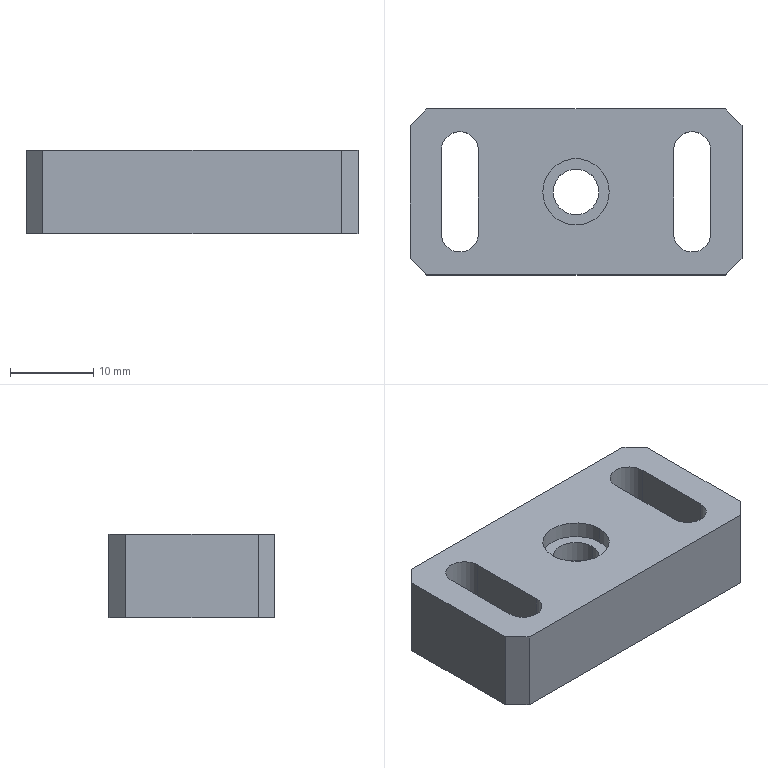Part | STEP file | 11-FG-B06611 | 1 solid | 36 faces | box 40 x 20 x 10 mm | volume 5422 mm3 | plane 22 | cylinder 14 | commonest cylinder face diameters 8 x6 4.5 x4 5.5 x2 10 x2
STEP:
#1=CARTESIAN_POINT('',(25.,-10.,5.4));
#2=VERTEX_POINT('',#1);
#3=CARTESIAN_POINT('',(15.,-10.,5.4));
#4=VERTEX_POINT('',#3);
#5=CARTESIAN_POINT('',(20.,-10.,5.4));
#6=DIRECTION('',(0.,0.,-1.));
#7=DIRECTION('',(-1.,0.,0.));
#8=AXIS2_PLACEMENT_3D('',#5,#6,#7);
#9=CIRCLE('',#8,5.);
#10=EDGE_CURVE('',#2,#4,#9,.T.);
#11=ORIENTED_EDGE('',*,*,#10,.F.);
#12=CARTESIAN_POINT('',(25.,-10.,0.));
#13=VERTEX_POINT('',#12);
#14=CARTESIAN_POINT('',(25.,-10.,0.));
#15=DIRECTION('',(0.,0.,-1.));
#16=VECTOR('',#15,1000.);
#17=LINE('',#14,#16);
#18=EDGE_CURVE('',#2,#13,#17,.T.);
#19=ORIENTED_EDGE('',*,*,#18,.T.);
#20=CARTESIAN_POINT('',(15.,-10.,0.));
#21=VERTEX_POINT('',#20);
#22=CARTESIAN_POINT('',(20.,-10.,0.));
#23=DIRECTION('',(0.,0.,-1.));
#24=DIRECTION('',(-1.,0.,0.));
#25=AXIS2_PLACEMENT_3D('',#22,#23,#24);
#26=CIRCLE('',#25,5.);
#27=EDGE_CURVE('',#13,#21,#26,.T.);
#28=ORIENTED_EDGE('',*,*,#27,.T.);
#29=CARTESIAN_POINT('',(15.,-10.,0.));
#30=DIRECTION('',(0.,0.,-1.));
#31=VECTOR('',#30,1000.);
#32=LINE('',#29,#31);
#33=EDGE_CURVE('',#4,#21,#32,.T.);
#34=ORIENTED_EDGE('',*,*,#33,.F.);
#35=EDGE_LOOP('',(#11,#19,#28,#34));
#36=FACE_OUTER_BOUND('',#35,.T.);
#37=CARTESIAN_POINT('',(20.,-10.,0.));
#38=DIRECTION('',(0.,0.,-1.));
#39=DIRECTION('',(-1.,0.,0.));
#40=AXIS2_PLACEMENT_3D('',#37,#38,#39);
#41=CYLINDRICAL_SURFACE('',#40,5.);
#42=ADVANCED_FACE('',(#36),#41,.F.);
#43=CARTESIAN_POINT('',(17.25,-10.,8.));
#44=VERTEX_POINT('',#43);
#45=CARTESIAN_POINT('',(22.75,-10.,8.));
#46=VERTEX_POINT('',#45);
#47=CARTESIAN_POINT('',(20.,-10.,8.));
#48=DIRECTION('',(0.,0.,1.));
#49=DIRECTION('',(1.,0.,0.));
#50=AXIS2_PLACEMENT_3D('',#47,#48,#49);
#51=CIRCLE('',#50,2.75);
#52=EDGE_CURVE('',#44,#46,#51,.T.);
#53=ORIENTED_EDGE('',*,*,#52,.T.);
#54=CARTESIAN_POINT('',(22.75,-10.,5.4));
#55=VERTEX_POINT('',#54);
#56=CARTESIAN_POINT('',(22.75,-10.,0.));
#57=DIRECTION('',(0.,0.,-1.));
#58=VECTOR('',#57,1000.);
#59=LINE('',#56,#58);
#60=EDGE_CURVE('',#46,#55,#59,.T.);
#61=ORIENTED_EDGE('',*,*,#60,.T.);
#62=CARTESIAN_POINT('',(17.25,-10.,5.4));
#63=VERTEX_POINT('',#62);
#64=CARTESIAN_POINT('',(20.,-10.,5.4));
#65=DIRECTION('',(0.,0.,-1.));
#66=DIRECTION('',(-1.,0.,0.));
#67=AXIS2_PLACEMENT_3D('',#64,#65,#66);
#68=CIRCLE('',#67,2.75);
#69=EDGE_CURVE('',#55,#63,#68,.T.);
#70=ORIENTED_EDGE('',*,*,#69,.T.);
#71=CARTESIAN_POINT('',(17.25,-10.,0.));
#72=DIRECTION('',(0.,0.,-1.));
#73=VECTOR('',#72,1000.);
#74=LINE('',#71,#73);
#75=EDGE_CURVE('',#44,#63,#74,.T.);
#76=ORIENTED_EDGE('',*,*,#75,.F.);
#77=EDGE_LOOP('',(#53,#61,#70,#76));
#78=FACE_OUTER_BOUND('',#77,.T.);
#79=CARTESIAN_POINT('',(20.,-10.,0.));
#80=DIRECTION('',(0.,0.,-1.));
#81=DIRECTION('',(-1.,0.,0.));
#82=AXIS2_PLACEMENT_3D('',#79,#80,#81);
#83=CYLINDRICAL_SURFACE('',#82,2.75);
#84=ADVANCED_FACE('',(#78),#83,.F.);
#85=CARTESIAN_POINT('',(16.,-10.,8.));
#86=VERTEX_POINT('',#85);
#87=CARTESIAN_POINT('',(24.,-10.,8.));
#88=VERTEX_POINT('',#87);
#89=CARTESIAN_POINT('',(20.,-10.,8.));
#90=DIRECTION('',(0.,0.,1.));
#91=DIRECTION('',(1.,0.,0.));
#92=AXIS2_PLACEMENT_3D('',#89,#90,#91);
#93=CIRCLE('',#92,4.);
#94=EDGE_CURVE('',#86,#88,#93,.T.);
#95=ORIENTED_EDGE('',*,*,#94,.F.);
#96=CARTESIAN_POINT('',(16.,-10.,10.));
#97=VERTEX_POINT('',#96);
#98=CARTESIAN_POINT('',(16.,-10.,8.));
#99=DIRECTION('',(0.,0.,1.));
#100=VECTOR('',#99,1000.);
#101=LINE('',#98,#100);
#102=EDGE_CURVE('',#86,#97,#101,.T.);
#103=ORIENTED_EDGE('',*,*,#102,.T.);
#104=CARTESIAN_POINT('',(24.,-10.,10.));
#105=VERTEX_POINT('',#104);
#106=CARTESIAN_POINT('',(20.,-10.,10.));
#107=DIRECTION('',(0.,0.,1.));
#108=DIRECTION('',(1.,0.,0.));
#109=AXIS2_PLACEMENT_3D('',#106,#107,#108);
#110=CIRCLE('',#109,4.);
#111=EDGE_CURVE('',#97,#105,#110,.T.);
#112=ORIENTED_EDGE('',*,*,#111,.T.);
#113=CARTESIAN_POINT('',(24.,-10.,8.));
#114=DIRECTION('',(0.,0.,1.));
#115=VECTOR('',#114,1000.);
#116=LINE('',#113,#115);
#117=EDGE_CURVE('',#88,#105,#116,.T.);
#118=ORIENTED_EDGE('',*,*,#117,.F.);
#119=EDGE_LOOP('',(#95,#103,#112,#118));
#120=FACE_OUTER_BOUND('',#119,.T.);
#121=CARTESIAN_POINT('',(20.,-10.,8.));
#122=DIRECTION('',(0.,0.,1.));
#123=DIRECTION('',(1.,0.,0.));
#124=AXIS2_PLACEMENT_3D('',#121,#122,#123);
#125=CYLINDRICAL_SURFACE('',#124,4.);
#126=ADVANCED_FACE('',(#120),#125,.F.);
#127=CARTESIAN_POINT('',(3.75,-15.,5.));
#128=VERTEX_POINT('',#127);
#129=CARTESIAN_POINT('',(8.25,-15.,5.));
#130=VERTEX_POINT('',#129);
#131=CARTESIAN_POINT('',(6.,-15.,5.));
#132=DIRECTION('',(0.,0.,1.));
#133=DIRECTION('',(-1.,0.,0.));
#134=AXIS2_PLACEMENT_3D('',#131,#132,#133);
#135=CIRCLE('',#134,2.25);
#136=EDGE_CURVE('',#128,#130,#135,.T.);
#137=ORIENTED_EDGE('',*,*,#136,.F.);
#138=CARTESIAN_POINT('',(3.75,-15.,10.));
#139=VERTEX_POINT('',#138);
#140=CARTESIAN_POINT('',(3.75,-15.,23.));
#141=DIRECTION('',(0.,0.,-1.));
#142=VECTOR('',#141,1000.);
#143=LINE('',#140,#142);
#144=EDGE_CURVE('',#139,#128,#143,.T.);
#145=ORIENTED_EDGE('',*,*,#144,.F.);
#146=CARTESIAN_POINT('',(8.25,-15.,10.));
#147=VERTEX_POINT('',#146);
#148=CARTESIAN_POINT('',(6.,-15.,10.));
#149=DIRECTION('',(0.,0.,1.));
#150=DIRECTION('',(1.,0.,0.));
#151=AXIS2_PLACEMENT_3D('',#148,#149,#150);
#152=CIRCLE('',#151,2.25);
#153=EDGE_CURVE('',#139,#147,#152,.T.);
#154=ORIENTED_EDGE('',*,*,#153,.T.);
#155=CARTESIAN_POINT('',(8.25,-15.,23.));
#156=DIRECTION('',(0.,0.,-1.));
#157=VECTOR('',#156,1000.);
#158=LINE('',#155,#157);
#159=EDGE_CURVE('',#147,#130,#158,.T.);
#160=ORIENTED_EDGE('',*,*,#159,.T.);
#161=EDGE_LOOP('',(#137,#145,#154,#160));
#162=FACE_OUTER_BOUND('',#161,.T.);
#163=CARTESIAN_POINT('',(6.,-15.,23.));
#164=DIRECTION('',(0.,0.,-1.));
#165=DIRECTION('',(-1.,0.,0.));
#166=AXIS2_PLACEMENT_3D('',#163,#164,#165);
#167=CYLINDRICAL_SURFACE('',#166,2.25);
#168=ADVANCED_FACE('',(#162),#167,.F.);
#169=CARTESIAN_POINT('',(8.25,-5.,5.));
#170=VERTEX_POINT('',#169);
#171=CARTESIAN_POINT('',(8.25,-15.,5.));
#172=DIRECTION('',(0.,1.,0.));
#173=VECTOR('',#172,1000.);
#174=LINE('',#171,#173);
#175=EDGE_CURVE('',#130,#170,#174,.T.);
#176=ORIENTED_EDGE('',*,*,#175,.F.);
#177=ORIENTED_EDGE('',*,*,#159,.F.);
#178=CARTESIAN_POINT('',(8.25,-5.,10.));
#179=VERTEX_POINT('',#178);
#180=CARTESIAN_POINT('',(8.25,-20.,10.));
#181=DIRECTION('',(0.,1.,0.));
#182=VECTOR('',#181,1000.);
#183=LINE('',#180,#182);
#184=EDGE_CURVE('',#147,#179,#183,.T.);
#185=ORIENTED_EDGE('',*,*,#184,.T.);
#186=CARTESIAN_POINT('',(8.25,-5.,23.));
#187=DIRECTION('',(0.,0.,-1.));
#188=VECTOR('',#187,1000.);
#189=LINE('',#186,#188);
#190=EDGE_CURVE('',#179,#170,#189,.T.);
#191=ORIENTED_EDGE('',*,*,#190,.T.);
#192=EDGE_LOOP('',(#176,#177,#185,#191));
#193=FACE_OUTER_BOUND('',#192,.T.);
#194=CARTESIAN_POINT('',(8.25,-15.,23.));
#195=DIRECTION('',(1.,0.,0.));
#196=DIRECTION('',(0.,1.,0.));
#197=AXIS2_PLACEMENT_3D('',#194,#195,#196);
#198=PLANE('',#197);
#199=ADVANCED_FACE('',(#193),#198,.F.);
#200=CARTESIAN_POINT('',(3.75,-5.,5.));
#201=VERTEX_POINT('',#200);
#202=CARTESIAN_POINT('',(6.,-5.,5.));
#203=DIRECTION('',(0.,0.,1.));
#204=DIRECTION('',(-1.,0.,0.));
#205=AXIS2_PLACEMENT_3D('',#202,#203,#204);
#206=CIRCLE('',#205,2.25);
#207=EDGE_CURVE('',#170,#201,#206,.T.);
#208=ORIENTED_EDGE('',*,*,#207,.F.);
#209=ORIENTED_EDGE('',*,*,#190,.F.);
#210=CARTESIAN_POINT('',(3.75,-5.,10.));
#211=VERTEX_POINT('',#210);
#212=CARTESIAN_POINT('',(6.,-5.,10.));
#213=DIRECTION('',(0.,0.,1.));
#214=DIRECTION('',(1.,0.,0.));
#215=AXIS2_PLACEMENT_3D('',#212,#213,#214);
#216=CIRCLE('',#215,2.25);
#217=EDGE_CURVE('',#179,#211,#216,.T.);
#218=ORIENTED_EDGE('',*,*,#217,.T.);
#219=CARTESIAN_POINT('',(3.75,-5.,23.));
#220=DIRECTION('',(0.,0.,-1.));
#221=VECTOR('',#220,1000.);
#222=LINE('',#219,#221);
#223=EDGE_CURVE('',#211,#201,#222,.T.);
#224=ORIENTED_EDGE('',*,*,#223,.T.);
#225=EDGE_LOOP('',(#208,#209,#218,#224));
#226=FACE_OUTER_BOUND('',#225,.T.);
#227=CARTESIAN_POINT('',(6.,-5.,23.));
#228=DIRECTION('',(0.,0.,-1.));
#229=DIRECTION('',(-1.,0.,0.));
#230=AXIS2_PLACEMENT_3D('',#227,#228,#229);
#231=CYLINDRICAL_SURFACE('',#230,2.25);
#232=ADVANCED_FACE('',(#226),#231,.F.);
#233=CARTESIAN_POINT('',(3.75,-15.,5.));
#234=DIRECTION('',(0.,-1.,0.));
#235=VECTOR('',#234,1000.);
#236=LINE('',#233,#235);
#237=EDGE_CURVE('',#201,#128,#236,.T.);
#238=ORIENTED_EDGE('',*,*,#237,.F.);
#239=ORIENTED_EDGE('',*,*,#223,.F.);
#240=CARTESIAN_POINT('',(3.75,-20.,10.));
#241=DIRECTION('',(0.,-1.,0.));
#242=VECTOR('',#241,1000.);
#243=LINE('',#240,#242);
#244=EDGE_CURVE('',#211,#139,#243,.T.);
#245=ORIENTED_EDGE('',*,*,#244,.T.);
#246=ORIENTED_EDGE('',*,*,#144,.T.);
#247=EDGE_LOOP('',(#238,#239,#245,#246));
#248=FACE_OUTER_BOUND('',#247,.T.);
#249=CARTESIAN_POINT('',(3.75,-15.,23.));
#250=DIRECTION('',(-1.,0.,0.));
#251=DIRECTION('',(0.,-1.,0.));
#252=AXIS2_PLACEMENT_3D('',#249,#250,#251);
#253=PLANE('',#252);
#254=ADVANCED_FACE('',(#248),#253,.F.);
#255=CARTESIAN_POINT('',(36.25,-15.,10.));
#256=VERTEX_POINT('',#255);
#257=CARTESIAN_POINT('',(36.25,-15.,5.));
#258=VERTEX_POINT('',#257);
#259=CARTESIAN_POINT('',(36.25,-15.,23.));
#260=DIRECTION('',(0.,0.,-1.));
#261=VECTOR('',#260,1000.);
#262=LINE('',#259,#261);
#263=EDGE_CURVE('',#256,#258,#262,.T.);
#264=ORIENTED_EDGE('',*,*,#263,.T.);
#265=CARTESIAN_POINT('',(31.75,-15.,5.));
#266=VERTEX_POINT('',#265);
#267=CARTESIAN_POINT('',(34.,-15.,5.));
#268=DIRECTION('',(0.,0.,-1.));
#269=DIRECTION('',(-1.,0.,0.));
#270=AXIS2_PLACEMENT_3D('',#267,#268,#269);
#271=CIRCLE('',#270,2.25);
#272=EDGE_CURVE('',#258,#266,#271,.T.);
#273=ORIENTED_EDGE('',*,*,#272,.T.);
#274=CARTESIAN_POINT('',(31.75,-15.,10.));
#275=VERTEX_POINT('',#274);
#276=CARTESIAN_POINT('',(31.75,-15.,23.));
#277=DIRECTION('',(0.,0.,-1.));
#278=VECTOR('',#277,1000.);
#279=LINE('',#276,#278);
#280=EDGE_CURVE('',#275,#266,#279,.T.);
#281=ORIENTED_EDGE('',*,*,#280,.F.);
#282=CARTESIAN_POINT('',(34.,-15.,10.));
#283=DIRECTION('',(0.,0.,-1.));
#284=DIRECTION('',(1.,0.,0.));
#285=AXIS2_PLACEMENT_3D('',#282,#283,#284);
#286=CIRCLE('',#285,2.25);
#287=EDGE_CURVE('',#256,#275,#286,.T.);
#288=ORIENTED_EDGE('',*,*,#287,.F.);
#289=EDGE_LOOP('',(#264,#273,#281,#288));
#290=FACE_OUTER_BOUND('',#289,.T.);
#291=CARTESIAN_POINT('',(34.,-15.,23.));
#292=DIRECTION('',(0.,0.,-1.));
#293=DIRECTION('',(-1.,0.,0.));
#294=AXIS2_PLACEMENT_3D('',#291,#292,#293);
#295=CYLINDRICAL_SURFACE('',#294,2.25);
#296=ADVANCED_FACE('',(#290),#295,.F.);
#297=CARTESIAN_POINT('',(36.25,-5.,10.));
#298=VERTEX_POINT('',#297);
#299=CARTESIAN_POINT('',(36.25,-5.,5.));
#300=VERTEX_POINT('',#299);
#301=CARTESIAN_POINT('',(36.25,-5.,23.));
#302=DIRECTION('',(0.,0.,-1.));
#303=VECTOR('',#302,1000.);
#304=LINE('',#301,#303);
#305=EDGE_CURVE('',#298,#300,#304,.T.);
#306=ORIENTED_EDGE('',*,*,#305,.T.);
#307=CARTESIAN_POINT('',(36.25,-15.,5.));
#308=DIRECTION('',(0.,-1.,0.));
#309=VECTOR('',#308,1000.);
#310=LINE('',#307,#309);
#311=EDGE_CURVE('',#300,#258,#310,.T.);
#312=ORIENTED_EDGE('',*,*,#311,.T.);
#313=ORIENTED_EDGE('',*,*,#263,.F.);
#314=CARTESIAN_POINT('',(36.25,-20.,10.));
#315=DIRECTION('',(0.,-1.,0.));
#316=VECTOR('',#315,1000.);
#317=LINE('',#314,#316);
#318=EDGE_CURVE('',#298,#256,#317,.T.);
#319=ORIENTED_EDGE('',*,*,#318,.F.);
#320=EDGE_LOOP('',(#306,#312,#313,#319));
#321=FACE_OUTER_BOUND('',#320,.T.);
#322=CARTESIAN_POINT('',(36.25,-15.,23.));
#323=DIRECTION('',(-1.,0.,0.));
#324=DIRECTION('',(0.,-1.,0.));
#325=AXIS2_PLACEMENT_3D('',#322,#323,#324);
#326=PLANE('',#325);
#327=ADVANCED_FACE('',(#321),#326,.T.);
#328=CARTESIAN_POINT('',(31.75,-5.,10.));
#329=VERTEX_POINT('',#328);
#330=CARTESIAN_POINT('',(31.75,-5.,5.));
#331=VERTEX_POINT('',#330);
#332=CARTESIAN_POINT('',(31.75,-5.,23.));
#333=DIRECTION('',(0.,0.,-1.));
#334=VECTOR('',#333,1000.);
#335=LINE('',#332,#334);
#336=EDGE_CURVE('',#329,#331,#335,.T.);
#337=ORIENTED_EDGE('',*,*,#336,.T.);
#338=CARTESIAN_POINT('',(34.,-5.,5.));
#339=DIRECTION('',(0.,0.,-1.));
#340=DIRECTION('',(-1.,0.,0.));
#341=AXIS2_PLACEMENT_3D('',#338,#339,#340);
#342=CIRCLE('',#341,2.25);
#343=EDGE_CURVE('',#331,#300,#342,.T.);
#344=ORIENTED_EDGE('',*,*,#343,.T.);
#345=ORIENTED_EDGE('',*,*,#305,.F.);
#346=CARTESIAN_POINT('',(34.,-5.,10.));
#347=DIRECTION('',(0.,0.,-1.));
#348=DIRECTION('',(1.,0.,0.));
#349=AXIS2_PLACEMENT_3D('',#346,#347,#348);
#350=CIRCLE('',#349,2.25);
#351=EDGE_CURVE('',#329,#298,#350,.T.);
#352=ORIENTED_EDGE('',*,*,#351,.F.);
#353=EDGE_LOOP('',(#337,#344,#345,#352));
#354=FACE_OUTER_BOUND('',#353,.T.);
#355=CARTESIAN_POINT('',(34.,-5.,23.));
#356=DIRECTION('',(0.,0.,-1.));
#357=DIRECTION('',(-1.,0.,0.));
#358=AXIS2_PLACEMENT_3D('',#355,#356,#357);
#359=CYLINDRICAL_SURFACE('',#358,2.25);
#360=ADVANCED_FACE('',(#354),#359,.F.);
#361=ORIENTED_EDGE('',*,*,#280,.T.);
#362=CARTESIAN_POINT('',(31.75,-15.,5.));
#363=DIRECTION('',(0.,1.,0.));
#364=VECTOR('',#363,1000.);
#365=LINE('',#362,#364);
#366=EDGE_CURVE('',#266,#331,#365,.T.);
#367=ORIENTED_EDGE('',*,*,#366,.T.);
#368=ORIENTED_EDGE('',*,*,#336,.F.);
#369=CARTESIAN_POINT('',(31.75,-20.,10.));
#370=DIRECTION('',(0.,1.,0.));
#371=VECTOR('',#370,1000.);
#372=LINE('',#369,#371);
#373=EDGE_CURVE('',#275,#329,#372,.T.);
#374=ORIENTED_EDGE('',*,*,#373,.F.);
#375=EDGE_LOOP('',(#361,#367,#368,#374));
#376=FACE_OUTER_BOUND('',#375,.T.);
#377=CARTESIAN_POINT('',(31.75,-15.,23.));
#378=DIRECTION('',(1.,0.,0.));
#379=DIRECTION('',(0.,1.,0.));
#380=AXIS2_PLACEMENT_3D('',#377,#378,#379);
#381=PLANE('',#380);
#382=ADVANCED_FACE('',(#376),#381,.T.);
#383=ORIENTED_EDGE('',*,*,#153,.F.);
#384=ORIENTED_EDGE('',*,*,#244,.F.);
#385=ORIENTED_EDGE('',*,*,#217,.F.);
#386=ORIENTED_EDGE('',*,*,#184,.F.);
#387=EDGE_LOOP('',(#383,#384,#385,#386));
#388=FACE_BOUND('',#387,.T.);
#389=CARTESIAN_POINT('',(20.,-10.,10.));
#390=DIRECTION('',(0.,0.,1.));
#391=DIRECTION('',(1.,0.,0.));
#392=AXIS2_PLACEMENT_3D('',#389,#390,#391);
#393=CIRCLE('',#392,4.);
#394=EDGE_CURVE('',#105,#97,#393,.T.);
#395=ORIENTED_EDGE('',*,*,#394,.F.);
#396=ORIENTED_EDGE('',*,*,#111,.F.);
#397=EDGE_LOOP('',(#395,#396));
#398=FACE_BOUND('',#397,.T.);
#399=CARTESIAN_POINT('',(0.,-2.,10.));
#400=VERTEX_POINT('',#399);
#401=CARTESIAN_POINT('',(0.,-18.,10.));
#402=VERTEX_POINT('',#401);
#403=CARTESIAN_POINT('',(0.,0.,10.));
#404=DIRECTION('',(0.,-1.,0.));
#405=VECTOR('',#404,1000.);
#406=LINE('',#403,#405);
#407=EDGE_CURVE('',#400,#402,#406,.T.);
#408=ORIENTED_EDGE('',*,*,#407,.T.);
#409=CARTESIAN_POINT('',(2.,-20.,10.));
#410=VERTEX_POINT('',#409);
#411=CARTESIAN_POINT('',(1.,-19.,10.));
#412=DIRECTION('',(0.7071,-0.7071,0.));
#413=VECTOR('',#412,1000.);
#414=LINE('',#411,#413);
#415=EDGE_CURVE('',#402,#410,#414,.T.);
#416=ORIENTED_EDGE('',*,*,#415,.T.);
#417=CARTESIAN_POINT('',(38.,-20.,10.));
#418=VERTEX_POINT('',#417);
#419=CARTESIAN_POINT('',(0.,-20.,10.));
#420=DIRECTION('',(1.,0.,0.));
#421=VECTOR('',#420,1000.);
#422=LINE('',#419,#421);
#423=EDGE_CURVE('',#410,#418,#422,.T.);
#424=ORIENTED_EDGE('',*,*,#423,.T.);
#425=CARTESIAN_POINT('',(40.,-18.,10.));
#426=VERTEX_POINT('',#425);
#427=CARTESIAN_POINT('',(19.,-39.,10.));
#428=DIRECTION('',(0.7071,0.7071,0.));
#429=VECTOR('',#428,1000.);
#430=LINE('',#427,#429);
#431=EDGE_CURVE('',#418,#426,#430,.T.);
#432=ORIENTED_EDGE('',*,*,#431,.T.);
#433=CARTESIAN_POINT('',(40.,-2.,10.));
#434=VERTEX_POINT('',#433);
#435=CARTESIAN_POINT('',(40.,0.,10.));
#436=DIRECTION('',(0.,1.,0.));
#437=VECTOR('',#436,1000.);
#438=LINE('',#435,#437);
#439=EDGE_CURVE('',#426,#434,#438,.T.);
#440=ORIENTED_EDGE('',*,*,#439,.T.);
#441=CARTESIAN_POINT('',(38.,0.,10.));
#442=VERTEX_POINT('',#441);
#443=CARTESIAN_POINT('',(29.,9.,10.));
#444=DIRECTION('',(-0.7071,0.7071,0.));
#445=VECTOR('',#444,1000.);
#446=LINE('',#443,#445);
#447=EDGE_CURVE('',#434,#442,#446,.T.);
#448=ORIENTED_EDGE('',*,*,#447,.T.);
#449=CARTESIAN_POINT('',(2.,0.,10.));
#450=VERTEX_POINT('',#449);
#451=CARTESIAN_POINT('',(0.,0.,10.));
#452=DIRECTION('',(-1.,0.,0.));
#453=VECTOR('',#452,1000.);
#454=LINE('',#451,#453);
#455=EDGE_CURVE('',#442,#450,#454,.T.);
#456=ORIENTED_EDGE('',*,*,#455,.T.);
#457=CARTESIAN_POINT('',(-9.,-11.,10.));
#458=DIRECTION('',(-0.7071,-0.7071,0.));
#459=VECTOR('',#458,1000.);
#460=LINE('',#457,#459);
#461=EDGE_CURVE('',#450,#400,#460,.T.);
#462=ORIENTED_EDGE('',*,*,#461,.T.);
#463=EDGE_LOOP('',(#408,#416,#424,#432,#440,#448,#456,#462));
#464=FACE_OUTER_BOUND('',#463,.T.);
#465=ORIENTED_EDGE('',*,*,#318,.T.);
#466=ORIENTED_EDGE('',*,*,#287,.T.);
#467=ORIENTED_EDGE('',*,*,#373,.T.);
#468=ORIENTED_EDGE('',*,*,#351,.T.);
#469=EDGE_LOOP('',(#465,#466,#467,#468));
#470=FACE_BOUND('',#469,.T.);
#471=CARTESIAN_POINT('',(0.,-20.,10.));
#472=DIRECTION('',(0.,0.,1.));
#473=DIRECTION('',(1.,0.,0.));
#474=AXIS2_PLACEMENT_3D('',#471,#472,#473);
#475=PLANE('',#474);
#476=ADVANCED_FACE('',(#388,#398,#464,#470),#475,.T.);
#477=CARTESIAN_POINT('',(10.,-5.,0.));
#478=VERTEX_POINT('',#477);
#479=CARTESIAN_POINT('',(10.,-15.,0.));
#480=VERTEX_POINT('',#479);
#481=CARTESIAN_POINT('',(10.,-5.,0.));
#482=DIRECTION('',(0.,-1.,0.));
#483=VECTOR('',#482,1000.);
#484=LINE('',#481,#483);
#485=EDGE_CURVE('',#478,#480,#484,.T.);
#486=ORIENTED_EDGE('',*,*,#485,.F.);
#487=CARTESIAN_POINT('',(2.,-5.,0.));
#488=VERTEX_POINT('',#487);
#489=CARTESIAN_POINT('',(6.,-5.,0.));
#490=DIRECTION('',(0.,0.,-1.));
#491=DIRECTION('',(-1.,0.,0.));
#492=AXIS2_PLACEMENT_3D('',#489,#490,#491);
#493=CIRCLE('',#492,4.);
#494=EDGE_CURVE('',#488,#478,#493,.T.);
#495=ORIENTED_EDGE('',*,*,#494,.F.);
#496=CARTESIAN_POINT('',(2.,-15.,0.));
#497=VERTEX_POINT('',#496);
#498=CARTESIAN_POINT('',(2.,-5.,0.));
#499=DIRECTION('',(0.,1.,0.));
#500=VECTOR('',#499,1000.);
#501=LINE('',#498,#500);
#502=EDGE_CURVE('',#497,#488,#501,.T.);
#503=ORIENTED_EDGE('',*,*,#502,.F.);
#504=CARTESIAN_POINT('',(6.,-15.,0.));
#505=DIRECTION('',(0.,0.,-1.));
#506=DIRECTION('',(-1.,0.,0.));
#507=AXIS2_PLACEMENT_3D('',#504,#505,#506);
#508=CIRCLE('',#507,4.);
#509=EDGE_CURVE('',#480,#497,#508,.T.);
#510=ORIENTED_EDGE('',*,*,#509,.F.);
#511=EDGE_LOOP('',(#486,#495,#503,#510));
#512=FACE_BOUND('',#511,.T.);
#513=CARTESIAN_POINT('',(38.,-5.,0.));
#514=VERTEX_POINT('',#513);
#515=CARTESIAN_POINT('',(38.,-15.,0.));
#516=VERTEX_POINT('',#515);
#517=CARTESIAN_POINT('',(38.,-5.,0.));
#518=DIRECTION('',(0.,-1.,0.));
#519=VECTOR('',#518,1000.);
#520=LINE('',#517,#519);
#521=EDGE_CURVE('',#514,#516,#520,.T.);
#522=ORIENTED_EDGE('',*,*,#521,.F.);
#523=CARTESIAN_POINT('',(30.,-5.,0.));
#524=VERTEX_POINT('',#523);
#525=CARTESIAN_POINT('',(34.,-5.,0.));
#526=DIRECTION('',(0.,0.,-1.));
#527=DIRECTION('',(-1.,0.,0.));
#528=AXIS2_PLACEMENT_3D('',#525,#526,#527);
#529=CIRCLE('',#528,4.);
#530=EDGE_CURVE('',#524,#514,#529,.T.);
#531=ORIENTED_EDGE('',*,*,#530,.F.);
#532=CARTESIAN_POINT('',(30.,-15.,0.));
#533=VERTEX_POINT('',#532);
#534=CARTESIAN_POINT('',(30.,-5.,0.));
#535=DIRECTION('',(0.,1.,0.));
#536=VECTOR('',#535,1000.);
#537=LINE('',#534,#536);
#538=EDGE_CURVE('',#533,#524,#537,.T.);
#539=ORIENTED_EDGE('',*,*,#538,.F.);
#540=CARTESIAN_POINT('',(34.,-15.,0.));
#541=DIRECTION('',(0.,0.,-1.));
#542=DIRECTION('',(-1.,0.,0.));
#543=AXIS2_PLACEMENT_3D('',#540,#541,#542);
#544=CIRCLE('',#543,4.);
#545=EDGE_CURVE('',#516,#533,#544,.T.);
#546=ORIENTED_EDGE('',*,*,#545,.F.);
#547=EDGE_LOOP('',(#522,#531,#539,#546));
#548=FACE_BOUND('',#547,.T.);
#549=CARTESIAN_POINT('',(2.,-20.,0.));
#550=VERTEX_POINT('',#549);
#551=CARTESIAN_POINT('',(38.,-20.,0.));
#552=VERTEX_POINT('',#551);
#553=CARTESIAN_POINT('',(0.,-20.,0.));
#554=DIRECTION('',(1.,0.,0.));
#555=VECTOR('',#554,1000.);
#556=LINE('',#553,#555);
#557=EDGE_CURVE('',#550,#552,#556,.T.);
#558=ORIENTED_EDGE('',*,*,#557,.F.);
#559=CARTESIAN_POINT('',(0.,-18.,0.));
#560=VERTEX_POINT('',#559);
#561=CARTESIAN_POINT('',(2.,-20.,0.));
#562=DIRECTION('',(-0.7071,0.7071,0.));
#563=VECTOR('',#562,1000.);
#564=LINE('',#561,#563);
#565=EDGE_CURVE('',#550,#560,#564,.T.);
#566=ORIENTED_EDGE('',*,*,#565,.T.);
#567=CARTESIAN_POINT('',(0.,-2.,0.));
#568=VERTEX_POINT('',#567);
#569=CARTESIAN_POINT('',(0.,0.,0.));
#570=DIRECTION('',(0.,-1.,0.));
#571=VECTOR('',#570,1000.);
#572=LINE('',#569,#571);
#573=EDGE_CURVE('',#568,#560,#572,.T.);
#574=ORIENTED_EDGE('',*,*,#573,.F.);
#575=CARTESIAN_POINT('',(2.,0.,0.));
#576=VERTEX_POINT('',#575);
#577=CARTESIAN_POINT('',(0.,-2.,0.));
#578=DIRECTION('',(0.7071,0.7071,0.));
#579=VECTOR('',#578,1000.);
#580=LINE('',#577,#579);
#581=EDGE_CURVE('',#568,#576,#580,.T.);
#582=ORIENTED_EDGE('',*,*,#581,.T.);
#583=CARTESIAN_POINT('',(38.,0.,0.));
#584=VERTEX_POINT('',#583);
#585=CARTESIAN_POINT('',(0.,0.,0.));
#586=DIRECTION('',(-1.,0.,0.));
#587=VECTOR('',#586,1000.);
#588=LINE('',#585,#587);
#589=EDGE_CURVE('',#584,#576,#588,.T.);
#590=ORIENTED_EDGE('',*,*,#589,.F.);
#591=CARTESIAN_POINT('',(40.,-2.,0.));
#592=VERTEX_POINT('',#591);
#593=CARTESIAN_POINT('',(38.,0.,0.));
#594=DIRECTION('',(0.7071,-0.7071,0.));
#595=VECTOR('',#594,1000.);
#596=LINE('',#593,#595);
#597=EDGE_CURVE('',#584,#592,#596,.T.);
#598=ORIENTED_EDGE('',*,*,#597,.T.);
#599=CARTESIAN_POINT('',(40.,-18.,0.));
#600=VERTEX_POINT('',#599);
#601=CARTESIAN_POINT('',(40.,0.,0.));
#602=DIRECTION('',(0.,1.,0.));
#603=VECTOR('',#602,1000.);
#604=LINE('',#601,#603);
#605=EDGE_CURVE('',#600,#592,#604,.T.);
#606=ORIENTED_EDGE('',*,*,#605,.F.);
#607=CARTESIAN_POINT('',(40.,-18.,0.));
#608=DIRECTION('',(-0.7071,-0.7071,0.));
#609=VECTOR('',#608,1000.);
#610=LINE('',#607,#609);
#611=EDGE_CURVE('',#600,#552,#610,.T.);
#612=ORIENTED_EDGE('',*,*,#611,.T.);
#613=EDGE_LOOP('',(#558,#566,#574,#582,#590,#598,#606,#612));
#614=FACE_OUTER_BOUND('',#613,.T.);
#615=CARTESIAN_POINT('',(20.,-10.,0.));
#616=DIRECTION('',(0.,0.,-1.));
#617=DIRECTION('',(-1.,0.,0.));
#618=AXIS2_PLACEMENT_3D('',#615,#616,#617);
#619=CIRCLE('',#618,5.);
#620=EDGE_CURVE('',#21,#13,#619,.T.);
#621=ORIENTED_EDGE('',*,*,#620,.F.);
#622=ORIENTED_EDGE('',*,*,#27,.F.);
#623=EDGE_LOOP('',(#621,#622));
#624=FACE_BOUND('',#623,.T.);
#625=CARTESIAN_POINT('',(0.,-20.,0.));
#626=DIRECTION('',(0.,0.,1.));
#627=DIRECTION('',(1.,0.,0.));
#628=AXIS2_PLACEMENT_3D('',#625,#626,#627);
#629=PLANE('',#628);
#630=ADVANCED_FACE('',(#512,#548,#614,#624),#629,.F.);
#631=ORIENTED_EDGE('',*,*,#573,.T.);
#632=CARTESIAN_POINT('',(0.,-18.,10.));
#633=DIRECTION('',(0.,0.,1.));
#634=VECTOR('',#633,1000.);
#635=LINE('',#632,#634);
#636=EDGE_CURVE('',#560,#402,#635,.T.);
#637=ORIENTED_EDGE('',*,*,#636,.T.);
#638=ORIENTED_EDGE('',*,*,#407,.F.);
#639=CARTESIAN_POINT('',(0.,-2.,10.));
#640=DIRECTION('',(0.,0.,-1.));
#641=VECTOR('',#640,1000.);
#642=LINE('',#639,#641);
#643=EDGE_CURVE('',#400,#568,#642,.T.);
#644=ORIENTED_EDGE('',*,*,#643,.T.);
#645=EDGE_LOOP('',(#631,#637,#638,#644));
#646=FACE_OUTER_BOUND('',#645,.T.);
#647=CARTESIAN_POINT('',(0.,0.,10.));
#648=DIRECTION('',(1.,0.,0.));
#649=DIRECTION('',(0.,1.,0.));
#650=AXIS2_PLACEMENT_3D('',#647,#648,#649);
#651=PLANE('',#650);
#652=ADVANCED_FACE('',(#646),#651,.F.);
#653=ORIENTED_EDGE('',*,*,#423,.F.);
#654=CARTESIAN_POINT('',(2.,-20.,10.));
#655=DIRECTION('',(0.,0.,-1.));
#656=VECTOR('',#655,1000.);
#657=LINE('',#654,#656);
#658=EDGE_CURVE('',#410,#550,#657,.T.);
#659=ORIENTED_EDGE('',*,*,#658,.T.);
#660=ORIENTED_EDGE('',*,*,#557,.T.);
#661=CARTESIAN_POINT('',(38.,-20.,10.));
#662=DIRECTION('',(0.,0.,1.));
#663=VECTOR('',#662,1000.);
#664=LINE('',#661,#663);
#665=EDGE_CURVE('',#552,#418,#664,.T.);
#666=ORIENTED_EDGE('',*,*,#665,.T.);
#667=EDGE_LOOP('',(#653,#659,#660,#666));
#668=FACE_OUTER_BOUND('',#667,.T.);
#669=CARTESIAN_POINT('',(0.,-20.,10.));
#670=DIRECTION('',(0.,1.,0.));
#671=DIRECTION('',(0.,0.,1.));
#672=AXIS2_PLACEMENT_3D('',#669,#670,#671);
#673=PLANE('',#672);
#674=ADVANCED_FACE('',(#668),#673,.F.);
#675=ORIENTED_EDGE('',*,*,#439,.F.);
#676=CARTESIAN_POINT('',(40.,-18.,10.));
#677=DIRECTION('',(0.,0.,-1.));
#678=VECTOR('',#677,1000.);
#679=LINE('',#676,#678);
#680=EDGE_CURVE('',#426,#600,#679,.T.);
#681=ORIENTED_EDGE('',*,*,#680,.T.);
#682=ORIENTED_EDGE('',*,*,#605,.T.);
#683=CARTESIAN_POINT('',(40.,-2.,10.));
#684=DIRECTION('',(0.,0.,1.));
#685=VECTOR('',#684,1000.);
#686=LINE('',#683,#685);
#687=EDGE_CURVE('',#592,#434,#686,.T.);
#688=ORIENTED_EDGE('',*,*,#687,.T.);
#689=EDGE_LOOP('',(#675,#681,#682,#688));
#690=FACE_OUTER_BOUND('',#689,.T.);
#691=CARTESIAN_POINT('',(40.,0.,10.));
#692=DIRECTION('',(-1.,0.,0.));
#693=DIRECTION('',(0.,0.,1.));
#694=AXIS2_PLACEMENT_3D('',#691,#692,#693);
#695=PLANE('',#694);
#696=ADVANCED_FACE('',(#690),#695,.F.);
#697=ORIENTED_EDGE('',*,*,#589,.T.);
#698=CARTESIAN_POINT('',(2.,0.,10.));
#699=DIRECTION('',(0.,0.,1.));
#700=VECTOR('',#699,1000.);
#701=LINE('',#698,#700);
#702=EDGE_CURVE('',#576,#450,#701,.T.);
#703=ORIENTED_EDGE('',*,*,#702,.T.);
#704=ORIENTED_EDGE('',*,*,#455,.F.);
#705=CARTESIAN_POINT('',(38.,0.,10.));
#706=DIRECTION('',(0.,0.,-1.));
#707=VECTOR('',#706,1000.);
#708=LINE('',#705,#707);
#709=EDGE_CURVE('',#442,#584,#708,.T.);
#710=ORIENTED_EDGE('',*,*,#709,.T.);
#711=EDGE_LOOP('',(#697,#703,#704,#710));
#712=FACE_OUTER_BOUND('',#711,.T.);
#713=CARTESIAN_POINT('',(0.,0.,10.));
#714=DIRECTION('',(0.,-1.,0.));
#715=DIRECTION('',(0.,0.,-1.));
#716=AXIS2_PLACEMENT_3D('',#713,#714,#715);
#717=PLANE('',#716);
#718=ADVANCED_FACE('',(#712),#717,.F.);
#719=ORIENTED_EDGE('',*,*,#102,.F.);
#720=CARTESIAN_POINT('',(20.,-10.,8.));
#721=DIRECTION('',(0.,0.,1.));
#722=DIRECTION('',(1.,0.,0.));
#723=AXIS2_PLACEMENT_3D('',#720,#721,#722);
#724=CIRCLE('',#723,4.);
#725=EDGE_CURVE('',#88,#86,#724,.T.);
#726=ORIENTED_EDGE('',*,*,#725,.F.);
#727=ORIENTED_EDGE('',*,*,#117,.T.);
#728=ORIENTED_EDGE('',*,*,#394,.T.);
#729=EDGE_LOOP('',(#719,#726,#727,#728));
#730=FACE_OUTER_BOUND('',#729,.T.);
#731=CARTESIAN_POINT('',(20.,-10.,8.));
#732=DIRECTION('',(0.,0.,1.));
#733=DIRECTION('',(1.,0.,0.));
#734=AXIS2_PLACEMENT_3D('',#731,#732,#733);
#735=CYLINDRICAL_SURFACE('',#734,4.);
#736=ADVANCED_FACE('',(#730),#735,.F.);
#737=ORIENTED_EDGE('',*,*,#52,.F.);
#738=CARTESIAN_POINT('',(20.,-10.,8.));
#739=DIRECTION('',(0.,0.,1.));
#740=DIRECTION('',(1.,0.,0.));
#741=AXIS2_PLACEMENT_3D('',#738,#739,#740);
#742=CIRCLE('',#741,2.75);
#743=EDGE_CURVE('',#46,#44,#742,.T.);
#744=ORIENTED_EDGE('',*,*,#743,.F.);
#745=EDGE_LOOP('',(#737,#744));
#746=FACE_BOUND('',#745,.T.);
#747=ORIENTED_EDGE('',*,*,#725,.T.);
#748=ORIENTED_EDGE('',*,*,#94,.T.);
#749=EDGE_LOOP('',(#747,#748));
#750=FACE_OUTER_BOUND('',#749,.T.);
#751=CARTESIAN_POINT('',(20.,-10.,8.));
#752=DIRECTION('',(0.,0.,1.));
#753=DIRECTION('',(1.,0.,0.));
#754=AXIS2_PLACEMENT_3D('',#751,#752,#753);
#755=PLANE('',#754);
#756=ADVANCED_FACE('',(#746,#750),#755,.T.);
#757=ORIENTED_EDGE('',*,*,#60,.F.);
#758=ORIENTED_EDGE('',*,*,#743,.T.);
#759=ORIENTED_EDGE('',*,*,#75,.T.);
#760=CARTESIAN_POINT('',(20.,-10.,5.4));
#761=DIRECTION('',(0.,0.,-1.));
#762=DIRECTION('',(-1.,0.,0.));
#763=AXIS2_PLACEMENT_3D('',#760,#761,#762);
#764=CIRCLE('',#763,2.75);
#765=EDGE_CURVE('',#63,#55,#764,.T.);
#766=ORIENTED_EDGE('',*,*,#765,.T.);
#767=EDGE_LOOP('',(#757,#758,#759,#766));
#768=FACE_OUTER_BOUND('',#767,.T.);
#769=CARTESIAN_POINT('',(20.,-10.,0.));
#770=DIRECTION('',(0.,0.,-1.));
#771=DIRECTION('',(-1.,0.,0.));
#772=AXIS2_PLACEMENT_3D('',#769,#770,#771);
#773=CYLINDRICAL_SURFACE('',#772,2.75);
#774=ADVANCED_FACE('',(#768),#773,.F.);
#775=ORIENTED_EDGE('',*,*,#765,.F.);
#776=ORIENTED_EDGE('',*,*,#69,.F.);
#777=EDGE_LOOP('',(#775,#776));
#778=FACE_BOUND('',#777,.T.);
#779=CARTESIAN_POINT('',(20.,-10.,5.4));
#780=DIRECTION('',(0.,0.,-1.));
#781=DIRECTION('',(-1.,0.,0.));
#782=AXIS2_PLACEMENT_3D('',#779,#780,#781);
#783=CIRCLE('',#782,5.);
#784=EDGE_CURVE('',#4,#2,#783,.T.);
#785=ORIENTED_EDGE('',*,*,#784,.T.);
#786=ORIENTED_EDGE('',*,*,#10,.T.);
#787=EDGE_LOOP('',(#785,#786));
#788=FACE_OUTER_BOUND('',#787,.T.);
#789=CARTESIAN_POINT('',(22.75,-10.,5.4));
#790=DIRECTION('',(0.,0.,1.));
#791=DIRECTION('',(1.,0.,0.));
#792=AXIS2_PLACEMENT_3D('',#789,#790,#791);
#793=PLANE('',#792);
#794=ADVANCED_FACE('',(#778,#788),#793,.F.);
#795=ORIENTED_EDGE('',*,*,#18,.F.);
#796=ORIENTED_EDGE('',*,*,#784,.F.);
#797=ORIENTED_EDGE('',*,*,#33,.T.);
#798=ORIENTED_EDGE('',*,*,#620,.T.);
#799=EDGE_LOOP('',(#795,#796,#797,#798));
#800=FACE_OUTER_BOUND('',#799,.T.);
#801=CARTESIAN_POINT('',(20.,-10.,0.));
#802=DIRECTION('',(0.,0.,-1.));
#803=DIRECTION('',(-1.,0.,0.));
#804=AXIS2_PLACEMENT_3D('',#801,#802,#803);
#805=CYLINDRICAL_SURFACE('',#804,5.);
#806=ADVANCED_FACE('',(#800),#805,.F.);
#807=ORIENTED_EDGE('',*,*,#530,.T.);
#808=CARTESIAN_POINT('',(38.,-5.,5.));
#809=VERTEX_POINT('',#808);
#810=CARTESIAN_POINT('',(38.,-5.,5.));
#811=DIRECTION('',(0.,0.,-1.));
#812=VECTOR('',#811,1000.);
#813=LINE('',#810,#812);
#814=EDGE_CURVE('',#809,#514,#813,.T.);
#815=ORIENTED_EDGE('',*,*,#814,.F.);
#816=CARTESIAN_POINT('',(30.,-5.,5.));
#817=VERTEX_POINT('',#816);
#818=CARTESIAN_POINT('',(34.,-5.,5.));
#819=DIRECTION('',(0.,0.,-1.));
#820=DIRECTION('',(-1.,0.,0.));
#821=AXIS2_PLACEMENT_3D('',#818,#819,#820);
#822=CIRCLE('',#821,4.);
#823=EDGE_CURVE('',#817,#809,#822,.T.);
#824=ORIENTED_EDGE('',*,*,#823,.F.);
#825=CARTESIAN_POINT('',(30.,-5.,5.));
#826=DIRECTION('',(0.,0.,-1.));
#827=VECTOR('',#826,1000.);
#828=LINE('',#825,#827);
#829=EDGE_CURVE('',#817,#524,#828,.T.);
#830=ORIENTED_EDGE('',*,*,#829,.T.);
#831=EDGE_LOOP('',(#807,#815,#824,#830));
#832=FACE_OUTER_BOUND('',#831,.T.);
#833=CARTESIAN_POINT('',(34.,-5.,5.));
#834=DIRECTION('',(0.,0.,-1.));
#835=DIRECTION('',(-1.,0.,0.));
#836=AXIS2_PLACEMENT_3D('',#833,#834,#835);
#837=CYLINDRICAL_SURFACE('',#836,4.);
#838=ADVANCED_FACE('',(#832),#837,.F.);
#839=ORIENTED_EDGE('',*,*,#538,.T.);
#840=ORIENTED_EDGE('',*,*,#829,.F.);
#841=CARTESIAN_POINT('',(30.,-15.,5.));
#842=VERTEX_POINT('',#841);
#843=CARTESIAN_POINT('',(30.,-5.,5.));
#844=DIRECTION('',(0.,1.,0.));
#845=VECTOR('',#844,1000.);
#846=LINE('',#843,#845);
#847=EDGE_CURVE('',#842,#817,#846,.T.);
#848=ORIENTED_EDGE('',*,*,#847,.F.);
#849=CARTESIAN_POINT('',(30.,-15.,5.));
#850=DIRECTION('',(0.,0.,-1.));
#851=VECTOR('',#850,1000.);
#852=LINE('',#849,#851);
#853=EDGE_CURVE('',#842,#533,#852,.T.);
#854=ORIENTED_EDGE('',*,*,#853,.T.);
#855=EDGE_LOOP('',(#839,#840,#848,#854));
#856=FACE_OUTER_BOUND('',#855,.T.);
#857=CARTESIAN_POINT('',(30.,-5.,5.));
#858=DIRECTION('',(-1.,0.,0.));
#859=DIRECTION('',(0.,0.,1.));
#860=AXIS2_PLACEMENT_3D('',#857,#858,#859);
#861=PLANE('',#860);
#862=ADVANCED_FACE('',(#856),#861,.F.);
#863=ORIENTED_EDGE('',*,*,#545,.T.);
#864=ORIENTED_EDGE('',*,*,#853,.F.);
#865=CARTESIAN_POINT('',(38.,-15.,5.));
#866=VERTEX_POINT('',#865);
#867=CARTESIAN_POINT('',(34.,-15.,5.));
#868=DIRECTION('',(0.,0.,-1.));
#869=DIRECTION('',(-1.,0.,0.));
#870=AXIS2_PLACEMENT_3D('',#867,#868,#869);
#871=CIRCLE('',#870,4.);
#872=EDGE_CURVE('',#866,#842,#871,.T.);
#873=ORIENTED_EDGE('',*,*,#872,.F.);
#874=CARTESIAN_POINT('',(38.,-15.,5.));
#875=DIRECTION('',(0.,0.,-1.));
#876=VECTOR('',#875,1000.);
#877=LINE('',#874,#876);
#878=EDGE_CURVE('',#866,#516,#877,.T.);
#879=ORIENTED_EDGE('',*,*,#878,.T.);
#880=EDGE_LOOP('',(#863,#864,#873,#879));
#881=FACE_OUTER_BOUND('',#880,.T.);
#882=CARTESIAN_POINT('',(34.,-15.,5.));
#883=DIRECTION('',(0.,0.,-1.));
#884=DIRECTION('',(-1.,0.,0.));
#885=AXIS2_PLACEMENT_3D('',#882,#883,#884);
#886=CYLINDRICAL_SURFACE('',#885,4.);
#887=ADVANCED_FACE('',(#881),#886,.F.);
#888=ORIENTED_EDGE('',*,*,#521,.T.);
#889=ORIENTED_EDGE('',*,*,#878,.F.);
#890=CARTESIAN_POINT('',(38.,-5.,5.));
#891=DIRECTION('',(0.,-1.,0.));
#892=VECTOR('',#891,1000.);
#893=LINE('',#890,#892);
#894=EDGE_CURVE('',#809,#866,#893,.T.);
#895=ORIENTED_EDGE('',*,*,#894,.F.);
#896=ORIENTED_EDGE('',*,*,#814,.T.);
#897=EDGE_LOOP('',(#888,#889,#895,#896));
#898=FACE_OUTER_BOUND('',#897,.T.);
#899=CARTESIAN_POINT('',(38.,-5.,5.));
#900=DIRECTION('',(1.,0.,0.));
#901=DIRECTION('',(0.,0.,-1.));
#902=AXIS2_PLACEMENT_3D('',#899,#900,#901);
#903=PLANE('',#902);
#904=ADVANCED_FACE('',(#898),#903,.F.);
#905=ORIENTED_EDGE('',*,*,#311,.F.);
#906=ORIENTED_EDGE('',*,*,#343,.F.);
#907=ORIENTED_EDGE('',*,*,#366,.F.);
#908=ORIENTED_EDGE('',*,*,#272,.F.);
#909=EDGE_LOOP('',(#905,#906,#907,#908));
#910=FACE_BOUND('',#909,.T.);
#911=ORIENTED_EDGE('',*,*,#823,.T.);
#912=ORIENTED_EDGE('',*,*,#894,.T.);
#913=ORIENTED_EDGE('',*,*,#872,.T.);
#914=ORIENTED_EDGE('',*,*,#847,.T.);
#915=EDGE_LOOP('',(#911,#912,#913,#914));
#916=FACE_OUTER_BOUND('',#915,.T.);
#917=CARTESIAN_POINT('',(34.,-5.,5.));
#918=DIRECTION('',(0.,0.,-1.));
#919=DIRECTION('',(-1.,0.,0.));
#920=AXIS2_PLACEMENT_3D('',#917,#918,#919);
#921=PLANE('',#920);
#922=ADVANCED_FACE('',(#910,#916),#921,.T.);
#923=CARTESIAN_POINT('',(2.,-5.,5.));
#924=VERTEX_POINT('',#923);
#925=CARTESIAN_POINT('',(10.,-5.,5.));
#926=VERTEX_POINT('',#925);
#927=CARTESIAN_POINT('',(6.,-5.,5.));
#928=DIRECTION('',(0.,0.,-1.));
#929=DIRECTION('',(-1.,0.,0.));
#930=AXIS2_PLACEMENT_3D('',#927,#928,#929);
#931=CIRCLE('',#930,4.);
#932=EDGE_CURVE('',#924,#926,#931,.T.);
#933=ORIENTED_EDGE('',*,*,#932,.T.);
#934=CARTESIAN_POINT('',(10.,-15.,5.));
#935=VERTEX_POINT('',#934);
#936=CARTESIAN_POINT('',(10.,-5.,5.));
#937=DIRECTION('',(0.,-1.,0.));
#938=VECTOR('',#937,1000.);
#939=LINE('',#936,#938);
#940=EDGE_CURVE('',#926,#935,#939,.T.);
#941=ORIENTED_EDGE('',*,*,#940,.T.);
#942=CARTESIAN_POINT('',(2.,-15.,5.));
#943=VERTEX_POINT('',#942);
#944=CARTESIAN_POINT('',(6.,-15.,5.));
#945=DIRECTION('',(0.,0.,-1.));
#946=DIRECTION('',(-1.,0.,0.));
#947=AXIS2_PLACEMENT_3D('',#944,#945,#946);
#948=CIRCLE('',#947,4.);
#949=EDGE_CURVE('',#935,#943,#948,.T.);
#950=ORIENTED_EDGE('',*,*,#949,.T.);
#951=CARTESIAN_POINT('',(2.,-5.,5.));
#952=DIRECTION('',(0.,1.,0.));
#953=VECTOR('',#952,1000.);
#954=LINE('',#951,#953);
#955=EDGE_CURVE('',#943,#924,#954,.T.);
#956=ORIENTED_EDGE('',*,*,#955,.T.);
#957=EDGE_LOOP('',(#933,#941,#950,#956));
#958=FACE_OUTER_BOUND('',#957,.T.);
#959=ORIENTED_EDGE('',*,*,#136,.T.);
#960=ORIENTED_EDGE('',*,*,#175,.T.);
#961=ORIENTED_EDGE('',*,*,#207,.T.);
#962=ORIENTED_EDGE('',*,*,#237,.T.);
#963=EDGE_LOOP('',(#959,#960,#961,#962));
#964=FACE_BOUND('',#963,.T.);
#965=CARTESIAN_POINT('',(6.,-5.,5.));
#966=DIRECTION('',(0.,0.,-1.));
#967=DIRECTION('',(-1.,0.,0.));
#968=AXIS2_PLACEMENT_3D('',#965,#966,#967);
#969=PLANE('',#968);
#970=ADVANCED_FACE('',(#958,#964),#969,.T.);
#971=ORIENTED_EDGE('',*,*,#494,.T.);
#972=CARTESIAN_POINT('',(10.,-5.,5.));
#973=DIRECTION('',(0.,0.,-1.));
#974=VECTOR('',#973,1000.);
#975=LINE('',#972,#974);
#976=EDGE_CURVE('',#926,#478,#975,.T.);
#977=ORIENTED_EDGE('',*,*,#976,.F.);
#978=ORIENTED_EDGE('',*,*,#932,.F.);
#979=CARTESIAN_POINT('',(2.,-5.,5.));
#980=DIRECTION('',(0.,0.,-1.));
#981=VECTOR('',#980,1000.);
#982=LINE('',#979,#981);
#983=EDGE_CURVE('',#924,#488,#982,.T.);
#984=ORIENTED_EDGE('',*,*,#983,.T.);
#985=EDGE_LOOP('',(#971,#977,#978,#984));
#986=FACE_OUTER_BOUND('',#985,.T.);
#987=CARTESIAN_POINT('',(6.,-5.,5.));
#988=DIRECTION('',(0.,0.,-1.));
#989=DIRECTION('',(-1.,0.,0.));
#990=AXIS2_PLACEMENT_3D('',#987,#988,#989);
#991=CYLINDRICAL_SURFACE('',#990,4.);
#992=ADVANCED_FACE('',(#986),#991,.F.);
#993=ORIENTED_EDGE('',*,*,#502,.T.);
#994=ORIENTED_EDGE('',*,*,#983,.F.);
#995=ORIENTED_EDGE('',*,*,#955,.F.);
#996=CARTESIAN_POINT('',(2.,-15.,5.));
#997=DIRECTION('',(0.,0.,-1.));
#998=VECTOR('',#997,1000.);
#999=LINE('',#996,#998);
#1000=EDGE_CURVE('',#943,#497,#999,.T.);
#1001=ORIENTED_EDGE('',*,*,#1000,.T.);
#1002=EDGE_LOOP('',(#993,#994,#995,#1001));
#1003=FACE_OUTER_BOUND('',#1002,.T.);
#1004=CARTESIAN_POINT('',(2.,-5.,5.));
#1005=DIRECTION('',(-1.,0.,0.));
#1006=DIRECTION('',(0.,-1.,0.));
#1007=AXIS2_PLACEMENT_3D('',#1004,#1005,#1006);
#1008=PLANE('',#1007);
#1009=ADVANCED_FACE('',(#1003),#1008,.F.);
#1010=ORIENTED_EDGE('',*,*,#509,.T.);
#1011=ORIENTED_EDGE('',*,*,#1000,.F.);
#1012=ORIENTED_EDGE('',*,*,#949,.F.);
#1013=CARTESIAN_POINT('',(10.,-15.,5.));
#1014=DIRECTION('',(0.,0.,-1.));
#1015=VECTOR('',#1014,1000.);
#1016=LINE('',#1013,#1015);
#1017=EDGE_CURVE('',#935,#480,#1016,.T.);
#1018=ORIENTED_EDGE('',*,*,#1017,.T.);
#1019=EDGE_LOOP('',(#1010,#1011,#1012,#1018));
#1020=FACE_OUTER_BOUND('',#1019,.T.);
#1021=CARTESIAN_POINT('',(6.,-15.,5.));
#1022=DIRECTION('',(0.,0.,-1.));
#1023=DIRECTION('',(-1.,0.,0.));
#1024=AXIS2_PLACEMENT_3D('',#1021,#1022,#1023);
#1025=CYLINDRICAL_SURFACE('',#1024,4.);
#1026=ADVANCED_FACE('',(#1020),#1025,.F.);
#1027=ORIENTED_EDGE('',*,*,#485,.T.);
#1028=ORIENTED_EDGE('',*,*,#1017,.F.);
#1029=ORIENTED_EDGE('',*,*,#940,.F.);
#1030=ORIENTED_EDGE('',*,*,#976,.T.);
#1031=EDGE_LOOP('',(#1027,#1028,#1029,#1030));
#1032=FACE_OUTER_BOUND('',#1031,.T.);
#1033=CARTESIAN_POINT('',(10.,-5.,5.));
#1034=DIRECTION('',(1.,0.,0.));
#1035=DIRECTION('',(0.,0.,-1.));
#1036=AXIS2_PLACEMENT_3D('',#1033,#1034,#1035);
#1037=PLANE('',#1036);
#1038=ADVANCED_FACE('',(#1032),#1037,.F.);
#1039=ORIENTED_EDGE('',*,*,#415,.F.);
#1040=ORIENTED_EDGE('',*,*,#636,.F.);
#1041=ORIENTED_EDGE('',*,*,#565,.F.);
#1042=ORIENTED_EDGE('',*,*,#658,.F.);
#1043=EDGE_LOOP('',(#1039,#1040,#1041,#1042));
#1044=FACE_OUTER_BOUND('',#1043,.T.);
#1045=CARTESIAN_POINT('',(2.,-20.,10.));
#1046=DIRECTION('',(0.7071,0.7071,0.));
#1047=DIRECTION('',(0.,0.,-1.));
#1048=AXIS2_PLACEMENT_3D('',#1045,#1046,#1047);
#1049=PLANE('',#1048);
#1050=ADVANCED_FACE('',(#1044),#1049,.F.);
#1051=ORIENTED_EDGE('',*,*,#431,.F.);
#1052=ORIENTED_EDGE('',*,*,#665,.F.);
#1053=ORIENTED_EDGE('',*,*,#611,.F.);
#1054=ORIENTED_EDGE('',*,*,#680,.F.);
#1055=EDGE_LOOP('',(#1051,#1052,#1053,#1054));
#1056=FACE_OUTER_BOUND('',#1055,.T.);
#1057=CARTESIAN_POINT('',(40.,-18.,10.));
#1058=DIRECTION('',(-0.7071,0.7071,0.));
#1059=DIRECTION('',(0.,0.,-1.));
#1060=AXIS2_PLACEMENT_3D('',#1057,#1058,#1059);
#1061=PLANE('',#1060);
#1062=ADVANCED_FACE('',(#1056),#1061,.F.);
#1063=ORIENTED_EDGE('',*,*,#461,.F.);
#1064=ORIENTED_EDGE('',*,*,#702,.F.);
#1065=ORIENTED_EDGE('',*,*,#581,.F.);
#1066=ORIENTED_EDGE('',*,*,#643,.F.);
#1067=EDGE_LOOP('',(#1063,#1064,#1065,#1066));
#1068=FACE_OUTER_BOUND('',#1067,.T.);
#1069=CARTESIAN_POINT('',(0.,-2.,10.));
#1070=DIRECTION('',(0.7071,-0.7071,0.));
#1071=DIRECTION('',(0.,0.,-1.));
#1072=AXIS2_PLACEMENT_3D('',#1069,#1070,#1071);
#1073=PLANE('',#1072);
#1074=ADVANCED_FACE('',(#1068),#1073,.F.);
#1075=ORIENTED_EDGE('',*,*,#447,.F.);
#1076=ORIENTED_EDGE('',*,*,#687,.F.);
#1077=ORIENTED_EDGE('',*,*,#597,.F.);
#1078=ORIENTED_EDGE('',*,*,#709,.F.);
#1079=EDGE_LOOP('',(#1075,#1076,#1077,#1078));
#1080=FACE_OUTER_BOUND('',#1079,.T.);
#1081=CARTESIAN_POINT('',(38.,0.,10.));
#1082=DIRECTION('',(-0.7071,-0.7071,0.));
#1083=DIRECTION('',(0.,0.,-1.));
#1084=AXIS2_PLACEMENT_3D('',#1081,#1082,#1083);
#1085=PLANE('',#1084);
#1086=ADVANCED_FACE('',(#1080),#1085,.F.);
#1087=CLOSED_SHELL('',(#42,#84,#126,#168,#199,#232,#254,#296,#327,#360,#382,#476,#630,#652,#674,#696,#718,#736,#756,#774,#794,#806,#838,#862,#887,#904,#922,#970,#992,#1009,#1026,#1038,#1050,#1062,#1074,#1086));
#1088=MANIFOLD_SOLID_BREP('',#1087);
#1089=CARTESIAN_POINT('',(0.,0.,0.));
#1090=DIRECTION('',(0.,0.,1.));
#1091=DIRECTION('',(1.,0.,0.));
#1092=AXIS2_PLACEMENT_3D('',#1089,#1090,#1091);
#1093=(LENGTH_UNIT()NAMED_UNIT(*)SI_UNIT(.MILLI.,.METRE.));
#1094=UNCERTAINTY_MEASURE_WITH_UNIT(LENGTH_MEASURE(0.00001),#1093,'','');
#1095=(NAMED_UNIT(*)PLANE_ANGLE_UNIT()SI_UNIT($,.RADIAN.));
#1096=(NAMED_UNIT(*)SI_UNIT($,.STERADIAN.)SOLID_ANGLE_UNIT());
#1097=(GEOMETRIC_REPRESENTATION_CONTEXT(3)GLOBAL_UNCERTAINTY_ASSIGNED_CONTEXT((#1094))GLOBAL_UNIT_ASSIGNED_CONTEXT((#1093,#1095,#1096))REPRESENTATION_CONTEXT('',''));
#1098=ADVANCED_BREP_SHAPE_REPRESENTATION('',(#1088,#1092),#1097);